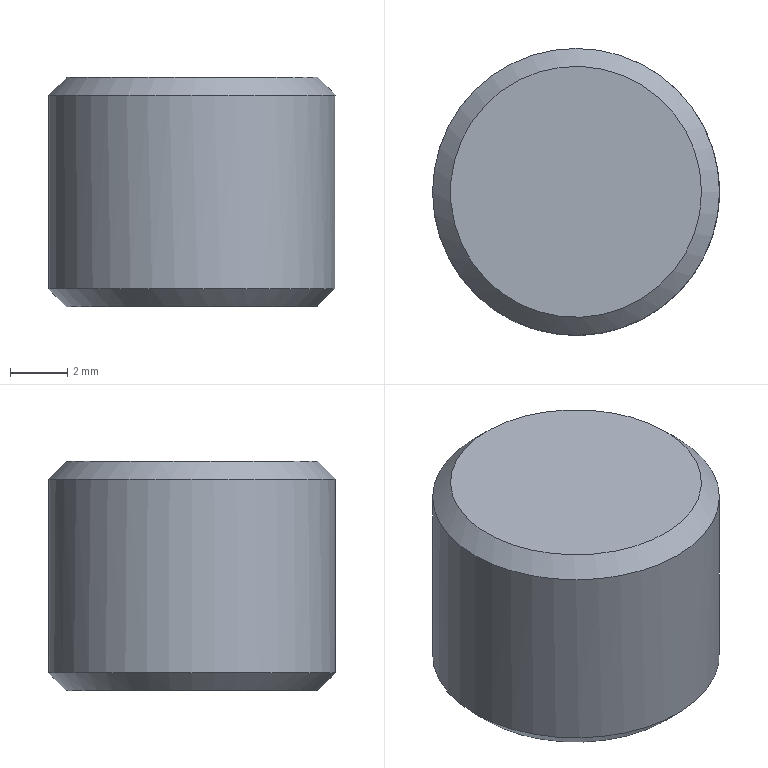Part | NX | features PG_666 2 | 1 solid | 5 faces | box 10 x 10 x 8 mm | volume 616.558 mm3 | plane 2 | cone 2 | cylinder 1 | commonest cylinder face diameters 10 x1
STEP:
#1=CARTESIAN_POINT('',(2819.722,-809.449,754.716));
#2=VERTEX_POINT('',#1);
#3=CARTESIAN_POINT('',(2824.097,-809.449,754.716));
#4=DIRECTION('',(0.,0.,-1.));
#5=DIRECTION('',(-1.,0.,0.));
#6=AXIS2_PLACEMENT_3D('',#3,#4,#5);
#7=CIRCLE('',#6,4.375);
#8=EDGE_CURVE('',#2,#2,#7,.T.);
#9=ORIENTED_EDGE('',*,*,#8,.T.);
#10=EDGE_LOOP('',(#9));
#11=FACE_BOUND('',#10,.T.);
#12=CARTESIAN_POINT('',(2824.097,-809.449,754.716));
#13=DIRECTION('',(0.,0.,-1.));
#14=DIRECTION('',(-1.,0.,0.));
#15=AXIS2_PLACEMENT_3D('',#12,#13,#14);
#16=PLANE('',#15);
#17=ADVANCED_FACE('',(#11),#16,.T.);
#18=CARTESIAN_POINT('',(2828.472,-809.449,762.716));
#19=VERTEX_POINT('',#18);
#20=CARTESIAN_POINT('',(2824.097,-809.449,762.716));
#21=DIRECTION('',(0.,0.,1.));
#22=DIRECTION('',(1.,0.,0.));
#23=AXIS2_PLACEMENT_3D('',#20,#21,#22);
#24=CIRCLE('',#23,4.375);
#25=EDGE_CURVE('',#19,#19,#24,.T.);
#26=ORIENTED_EDGE('',*,*,#25,.T.);
#27=EDGE_LOOP('',(#26));
#28=FACE_BOUND('',#27,.T.);
#29=CARTESIAN_POINT('',(2824.097,-809.449,762.716));
#30=DIRECTION('',(0.,0.,1.));
#31=DIRECTION('',(1.,0.,0.));
#32=AXIS2_PLACEMENT_3D('',#29,#30,#31);
#33=PLANE('',#32);
#34=ADVANCED_FACE('',(#28),#33,.T.);
#35=CARTESIAN_POINT('',(2829.097,-809.449,762.091));
#36=VERTEX_POINT('',#35);
#37=CARTESIAN_POINT('',(2824.097,-809.449,762.091));
#38=DIRECTION('',(0.,0.,1.));
#39=DIRECTION('',(1.,0.,0.));
#40=AXIS2_PLACEMENT_3D('',#37,#38,#39);
#41=CIRCLE('',#40,5.);
#42=EDGE_CURVE('',#36,#36,#41,.F.);
#43=ORIENTED_EDGE('',*,*,#42,.T.);
#44=EDGE_LOOP('',(#43));
#45=FACE_BOUND('',#44,.T.);
#46=CARTESIAN_POINT('',(2819.097,-809.449,755.341));
#47=VERTEX_POINT('',#46);
#48=CARTESIAN_POINT('',(2824.097,-809.449,755.341));
#49=DIRECTION('',(0.,0.,-1.));
#50=DIRECTION('',(-1.,0.,0.));
#51=AXIS2_PLACEMENT_3D('',#48,#49,#50);
#52=CIRCLE('',#51,5.);
#53=EDGE_CURVE('',#47,#47,#52,.F.);
#54=ORIENTED_EDGE('',*,*,#53,.T.);
#55=EDGE_LOOP('',(#54));
#56=FACE_BOUND('',#55,.T.);
#57=CARTESIAN_POINT('',(2824.097,-809.449,823.716));
#58=DIRECTION('',(0.,0.,-1.));
#59=DIRECTION('',(-1.,0.,0.));
#60=AXIS2_PLACEMENT_3D('',#57,#58,#59);
#61=CYLINDRICAL_SURFACE('',#60,5.);
#62=ADVANCED_FACE('',(#45,#56),#61,.T.);
#63=ORIENTED_EDGE('',*,*,#25,.F.);
#64=EDGE_LOOP('',(#63));
#65=FACE_BOUND('',#64,.T.);
#66=ORIENTED_EDGE('',*,*,#42,.F.);
#67=EDGE_LOOP('',(#66));
#68=FACE_BOUND('',#67,.T.);
#69=CARTESIAN_POINT('',(2824.097,-809.449,762.091));
#70=DIRECTION('',(0.,0.,-1.));
#71=DIRECTION('',(-1.,0.,0.));
#72=AXIS2_PLACEMENT_3D('',#69,#70,#71);
#73=CONICAL_SURFACE('',#72,5.,0.7854);
#74=ADVANCED_FACE('',(#65,#68),#73,.T.);
#75=ORIENTED_EDGE('',*,*,#8,.F.);
#76=EDGE_LOOP('',(#75));
#77=FACE_BOUND('',#76,.T.);
#78=ORIENTED_EDGE('',*,*,#53,.F.);
#79=EDGE_LOOP('',(#78));
#80=FACE_BOUND('',#79,.T.);
#81=CARTESIAN_POINT('',(2824.097,-809.449,755.341));
#82=DIRECTION('',(0.,0.,1.));
#83=DIRECTION('',(1.,0.,0.));
#84=AXIS2_PLACEMENT_3D('',#81,#82,#83);
#85=CONICAL_SURFACE('',#84,5.,0.7854);
#86=ADVANCED_FACE('',(#77,#80),#85,.T.);
#87=CLOSED_SHELL('',(#17,#34,#62,#74,#86));
#88=MANIFOLD_SOLID_BREP('',#87);
#89=(LENGTH_UNIT()NAMED_UNIT(*)SI_UNIT(.MILLI.,.METRE.));
#90=UNCERTAINTY_MEASURE_WITH_UNIT(LENGTH_MEASURE(0.00001),#89,'','');
#91=(NAMED_UNIT(*)PLANE_ANGLE_UNIT()SI_UNIT($,.RADIAN.));
#92=(NAMED_UNIT(*)SI_UNIT($,.STERADIAN.)SOLID_ANGLE_UNIT());
#93=(GEOMETRIC_REPRESENTATION_CONTEXT(3)GLOBAL_UNCERTAINTY_ASSIGNED_CONTEXT((#90))GLOBAL_UNIT_ASSIGNED_CONTEXT((#89,#91,#92))REPRESENTATION_CONTEXT('',''));
#94=ADVANCED_BREP_SHAPE_REPRESENTATION('',(#88),#93);